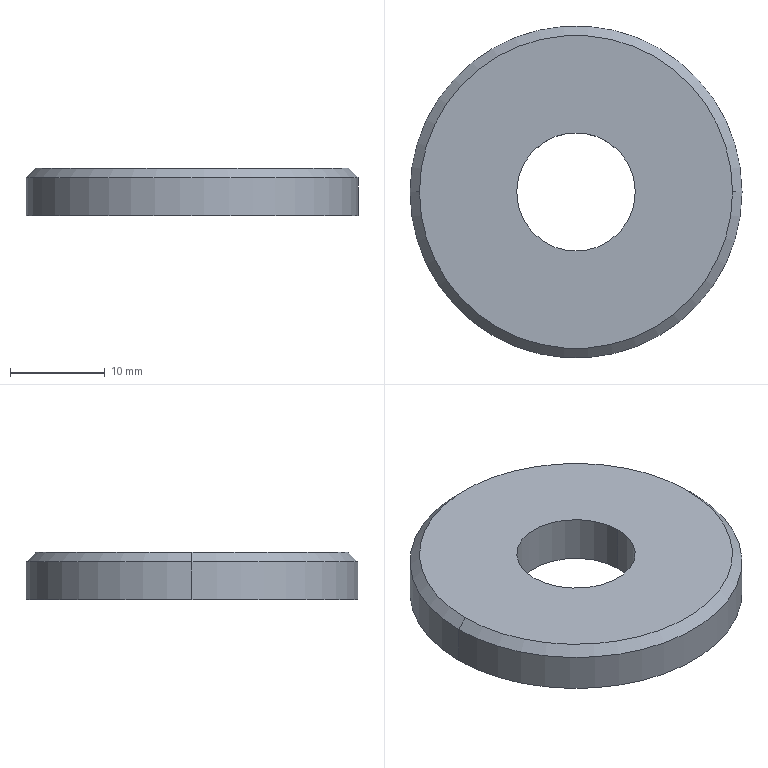Part | SolidWorks | features Revolution 1 | 1 solid | 8 faces | box 35 x 35 x 5 mm | volume 4143 mm3 | cylinder 4 | cone 2 | plane 2 | commonest cylinder face diameters 12.5 x2 35 x2
STEP:
#1=CARTESIAN_POINT('',(-16.5,0.,2.5));
#2=VERTEX_POINT('',#1);
#3=CARTESIAN_POINT('',(16.5,0.,2.5));
#4=VERTEX_POINT('',#3);
#5=CARTESIAN_POINT('',(0.,0.,2.5));
#6=DIRECTION('',(0.,0.,-1.));
#7=DIRECTION('',(-1.,0.,0.));
#8=AXIS2_PLACEMENT_3D('',#5,#6,#7);
#9=CIRCLE('',#8,16.5);
#10=EDGE_CURVE('',#2,#4,#9,.T.);
#11=ORIENTED_EDGE('',*,*,#10,.T.);
#12=CARTESIAN_POINT('',(17.5,0.,1.5));
#13=VERTEX_POINT('',#12);
#14=CARTESIAN_POINT('',(17.5,0.,1.5));
#15=DIRECTION('',(0.7071,0.,-0.7071));
#16=VECTOR('',#15,1000.);
#17=LINE('',#14,#16);
#18=EDGE_CURVE('',#4,#13,#17,.T.);
#19=ORIENTED_EDGE('',*,*,#18,.T.);
#20=CARTESIAN_POINT('',(-17.5,0.,1.5));
#21=VERTEX_POINT('',#20);
#22=CARTESIAN_POINT('',(0.,0.,1.5));
#23=DIRECTION('',(0.,0.,-1.));
#24=DIRECTION('',(-1.,0.,0.));
#25=AXIS2_PLACEMENT_3D('',#22,#23,#24);
#26=CIRCLE('',#25,17.5);
#27=EDGE_CURVE('',#21,#13,#26,.T.);
#28=ORIENTED_EDGE('',*,*,#27,.F.);
#29=CARTESIAN_POINT('',(-17.5,0.,1.5));
#30=DIRECTION('',(-0.7071,0.,-0.7071));
#31=VECTOR('',#30,1000.);
#32=LINE('',#29,#31);
#33=EDGE_CURVE('',#2,#21,#32,.T.);
#34=ORIENTED_EDGE('',*,*,#33,.F.);
#35=EDGE_LOOP('',(#11,#19,#28,#34));
#36=FACE_OUTER_BOUND('',#35,.T.);
#37=CARTESIAN_POINT('',(0.,0.,1.5));
#38=DIRECTION('',(0.,0.,-1.));
#39=DIRECTION('',(-1.,0.,0.));
#40=AXIS2_PLACEMENT_3D('',#37,#38,#39);
#41=CONICAL_SURFACE('',#40,17.5,0.7854);
#42=ADVANCED_FACE('',(#36),#41,.T.);
#43=ORIENTED_EDGE('',*,*,#27,.T.);
#44=CARTESIAN_POINT('',(17.5,0.,-2.5));
#45=VERTEX_POINT('',#44);
#46=CARTESIAN_POINT('',(17.5,0.,2.5));
#47=DIRECTION('',(0.,0.,-1.));
#48=VECTOR('',#47,1000.);
#49=LINE('',#46,#48);
#50=EDGE_CURVE('',#13,#45,#49,.T.);
#51=ORIENTED_EDGE('',*,*,#50,.T.);
#52=CARTESIAN_POINT('',(-17.5,0.,-2.5));
#53=VERTEX_POINT('',#52);
#54=CARTESIAN_POINT('',(0.,0.,-2.5));
#55=DIRECTION('',(0.,0.,-1.));
#56=DIRECTION('',(-1.,0.,0.));
#57=AXIS2_PLACEMENT_3D('',#54,#55,#56);
#58=CIRCLE('',#57,17.5);
#59=EDGE_CURVE('',#53,#45,#58,.T.);
#60=ORIENTED_EDGE('',*,*,#59,.F.);
#61=CARTESIAN_POINT('',(-17.5,0.,2.5));
#62=DIRECTION('',(0.,0.,-1.));
#63=VECTOR('',#62,1000.);
#64=LINE('',#61,#63);
#65=EDGE_CURVE('',#21,#53,#64,.T.);
#66=ORIENTED_EDGE('',*,*,#65,.F.);
#67=EDGE_LOOP('',(#43,#51,#60,#66));
#68=FACE_OUTER_BOUND('',#67,.T.);
#69=CARTESIAN_POINT('',(0.,0.,2.5));
#70=DIRECTION('',(0.,0.,-1.));
#71=DIRECTION('',(-1.,0.,0.));
#72=AXIS2_PLACEMENT_3D('',#69,#70,#71);
#73=CYLINDRICAL_SURFACE('',#72,17.5);
#74=ADVANCED_FACE('',(#68),#73,.T.);
#75=CARTESIAN_POINT('',(6.25,0.,2.5));
#76=VERTEX_POINT('',#75);
#77=CARTESIAN_POINT('',(-6.25,0.,2.5));
#78=VERTEX_POINT('',#77);
#79=CARTESIAN_POINT('',(0.,0.,2.5));
#80=DIRECTION('',(0.,0.,-1.));
#81=DIRECTION('',(-1.,0.,0.));
#82=AXIS2_PLACEMENT_3D('',#79,#80,#81);
#83=CIRCLE('',#82,6.25);
#84=EDGE_CURVE('',#76,#78,#83,.T.);
#85=ORIENTED_EDGE('',*,*,#84,.F.);
#86=CARTESIAN_POINT('',(6.25,0.,-2.5));
#87=VERTEX_POINT('',#86);
#88=CARTESIAN_POINT('',(6.25,0.,2.5));
#89=DIRECTION('',(0.,0.,-1.));
#90=VECTOR('',#89,1000.);
#91=LINE('',#88,#90);
#92=EDGE_CURVE('',#76,#87,#91,.T.);
#93=ORIENTED_EDGE('',*,*,#92,.T.);
#94=CARTESIAN_POINT('',(-6.25,0.,-2.5));
#95=VERTEX_POINT('',#94);
#96=CARTESIAN_POINT('',(0.,0.,-2.5));
#97=DIRECTION('',(0.,0.,-1.));
#98=DIRECTION('',(-1.,0.,0.));
#99=AXIS2_PLACEMENT_3D('',#96,#97,#98);
#100=CIRCLE('',#99,6.25);
#101=EDGE_CURVE('',#87,#95,#100,.T.);
#102=ORIENTED_EDGE('',*,*,#101,.T.);
#103=CARTESIAN_POINT('',(-6.25,0.,2.5));
#104=DIRECTION('',(0.,0.,-1.));
#105=VECTOR('',#104,1000.);
#106=LINE('',#103,#105);
#107=EDGE_CURVE('',#78,#95,#106,.T.);
#108=ORIENTED_EDGE('',*,*,#107,.F.);
#109=EDGE_LOOP('',(#85,#93,#102,#108));
#110=FACE_OUTER_BOUND('',#109,.T.);
#111=CARTESIAN_POINT('',(0.,0.,2.5));
#112=DIRECTION('',(0.,0.,-1.));
#113=DIRECTION('',(-1.,0.,0.));
#114=AXIS2_PLACEMENT_3D('',#111,#112,#113);
#115=CYLINDRICAL_SURFACE('',#114,6.25);
#116=ADVANCED_FACE('',(#110),#115,.F.);
#117=CARTESIAN_POINT('',(0.,0.,2.5));
#118=DIRECTION('',(0.,0.,-1.));
#119=DIRECTION('',(-1.,0.,0.));
#120=AXIS2_PLACEMENT_3D('',#117,#118,#119);
#121=CIRCLE('',#120,6.25);
#122=EDGE_CURVE('',#78,#76,#121,.T.);
#123=ORIENTED_EDGE('',*,*,#122,.T.);
#124=ORIENTED_EDGE('',*,*,#84,.T.);
#125=EDGE_LOOP('',(#123,#124));
#126=FACE_BOUND('',#125,.T.);
#127=ORIENTED_EDGE('',*,*,#10,.F.);
#128=CARTESIAN_POINT('',(0.,0.,2.5));
#129=DIRECTION('',(0.,0.,-1.));
#130=DIRECTION('',(-1.,0.,0.));
#131=AXIS2_PLACEMENT_3D('',#128,#129,#130);
#132=CIRCLE('',#131,16.5);
#133=EDGE_CURVE('',#4,#2,#132,.T.);
#134=ORIENTED_EDGE('',*,*,#133,.F.);
#135=EDGE_LOOP('',(#127,#134));
#136=FACE_OUTER_BOUND('',#135,.T.);
#137=CARTESIAN_POINT('',(16.5,0.,2.5));
#138=DIRECTION('',(0.,0.,1.));
#139=DIRECTION('',(1.,0.,0.));
#140=AXIS2_PLACEMENT_3D('',#137,#138,#139);
#141=PLANE('',#140);
#142=ADVANCED_FACE('',(#126,#136),#141,.T.);
#143=ORIENTED_EDGE('',*,*,#92,.F.);
#144=ORIENTED_EDGE('',*,*,#122,.F.);
#145=ORIENTED_EDGE('',*,*,#107,.T.);
#146=CARTESIAN_POINT('',(0.,0.,-2.5));
#147=DIRECTION('',(0.,0.,-1.));
#148=DIRECTION('',(-1.,0.,0.));
#149=AXIS2_PLACEMENT_3D('',#146,#147,#148);
#150=CIRCLE('',#149,6.25);
#151=EDGE_CURVE('',#95,#87,#150,.T.);
#152=ORIENTED_EDGE('',*,*,#151,.T.);
#153=EDGE_LOOP('',(#143,#144,#145,#152));
#154=FACE_OUTER_BOUND('',#153,.T.);
#155=CARTESIAN_POINT('',(0.,0.,2.5));
#156=DIRECTION('',(0.,0.,-1.));
#157=DIRECTION('',(-1.,0.,0.));
#158=AXIS2_PLACEMENT_3D('',#155,#156,#157);
#159=CYLINDRICAL_SURFACE('',#158,6.25);
#160=ADVANCED_FACE('',(#154),#159,.F.);
#161=ORIENTED_EDGE('',*,*,#59,.T.);
#162=CARTESIAN_POINT('',(0.,0.,-2.5));
#163=DIRECTION('',(0.,0.,-1.));
#164=DIRECTION('',(-1.,0.,0.));
#165=AXIS2_PLACEMENT_3D('',#162,#163,#164);
#166=CIRCLE('',#165,17.5);
#167=EDGE_CURVE('',#45,#53,#166,.T.);
#168=ORIENTED_EDGE('',*,*,#167,.T.);
#169=EDGE_LOOP('',(#161,#168));
#170=FACE_OUTER_BOUND('',#169,.T.);
#171=ORIENTED_EDGE('',*,*,#151,.F.);
#172=ORIENTED_EDGE('',*,*,#101,.F.);
#173=EDGE_LOOP('',(#171,#172));
#174=FACE_BOUND('',#173,.T.);
#175=CARTESIAN_POINT('',(6.25,0.,-2.5));
#176=DIRECTION('',(0.,0.,-1.));
#177=DIRECTION('',(-1.,0.,0.));
#178=AXIS2_PLACEMENT_3D('',#175,#176,#177);
#179=PLANE('',#178);
#180=ADVANCED_FACE('',(#170,#174),#179,.T.);
#181=ORIENTED_EDGE('',*,*,#50,.F.);
#182=CARTESIAN_POINT('',(0.,0.,1.5));
#183=DIRECTION('',(0.,0.,-1.));
#184=DIRECTION('',(-1.,0.,0.));
#185=AXIS2_PLACEMENT_3D('',#182,#183,#184);
#186=CIRCLE('',#185,17.5);
#187=EDGE_CURVE('',#13,#21,#186,.T.);
#188=ORIENTED_EDGE('',*,*,#187,.T.);
#189=ORIENTED_EDGE('',*,*,#65,.T.);
#190=ORIENTED_EDGE('',*,*,#167,.F.);
#191=EDGE_LOOP('',(#181,#188,#189,#190));
#192=FACE_OUTER_BOUND('',#191,.T.);
#193=CARTESIAN_POINT('',(0.,0.,2.5));
#194=DIRECTION('',(0.,0.,-1.));
#195=DIRECTION('',(-1.,0.,0.));
#196=AXIS2_PLACEMENT_3D('',#193,#194,#195);
#197=CYLINDRICAL_SURFACE('',#196,17.5);
#198=ADVANCED_FACE('',(#192),#197,.T.);
#199=ORIENTED_EDGE('',*,*,#18,.F.);
#200=ORIENTED_EDGE('',*,*,#133,.T.);
#201=ORIENTED_EDGE('',*,*,#33,.T.);
#202=ORIENTED_EDGE('',*,*,#187,.F.);
#203=EDGE_LOOP('',(#199,#200,#201,#202));
#204=FACE_OUTER_BOUND('',#203,.T.);
#205=CARTESIAN_POINT('',(0.,0.,1.5));
#206=DIRECTION('',(0.,0.,-1.));
#207=DIRECTION('',(-1.,0.,0.));
#208=AXIS2_PLACEMENT_3D('',#205,#206,#207);
#209=CONICAL_SURFACE('',#208,17.5,0.7854);
#210=ADVANCED_FACE('',(#204),#209,.T.);
#211=CLOSED_SHELL('',(#42,#74,#116,#142,#160,#180,#198,#210));
#212=MANIFOLD_SOLID_BREP('',#211);
#213=CARTESIAN_POINT('',(0.,0.,0.));
#214=DIRECTION('',(0.,0.,1.));
#215=DIRECTION('',(1.,0.,0.));
#216=AXIS2_PLACEMENT_3D('',#213,#214,#215);
#217=(LENGTH_UNIT()NAMED_UNIT(*)SI_UNIT(.MILLI.,.METRE.));
#218=UNCERTAINTY_MEASURE_WITH_UNIT(LENGTH_MEASURE(0.00001),#217,'','');
#219=(NAMED_UNIT(*)PLANE_ANGLE_UNIT()SI_UNIT($,.RADIAN.));
#220=(NAMED_UNIT(*)SI_UNIT($,.STERADIAN.)SOLID_ANGLE_UNIT());
#221=(GEOMETRIC_REPRESENTATION_CONTEXT(3)GLOBAL_UNCERTAINTY_ASSIGNED_CONTEXT((#218))GLOBAL_UNIT_ASSIGNED_CONTEXT((#217,#219,#220))REPRESENTATION_CONTEXT('',''));
#222=ADVANCED_BREP_SHAPE_REPRESENTATION('',(#212,#216),#221);